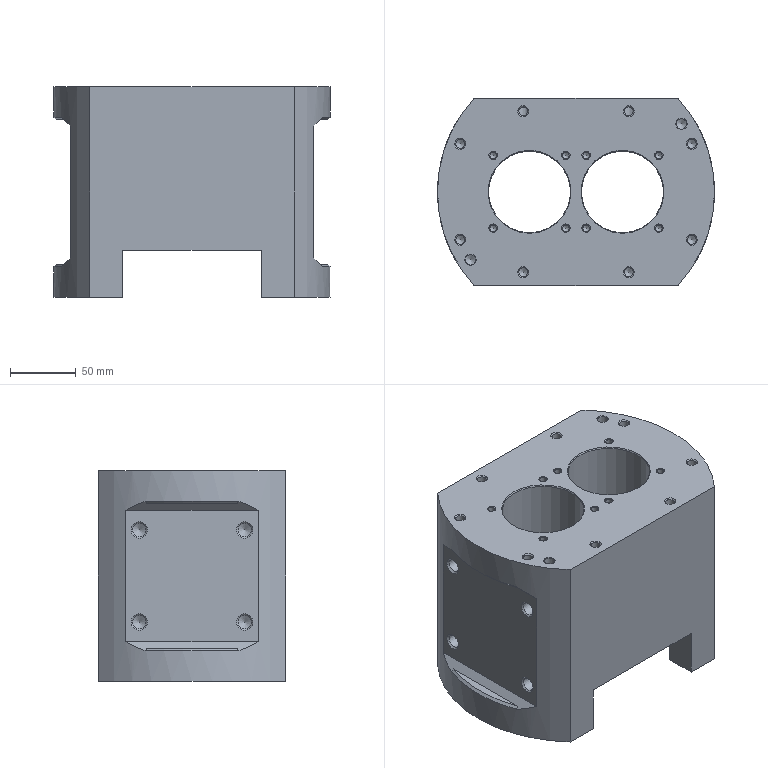NC program | NX | posted with a generic post | part box 210 x 142 x 160 mm
Lines 1 to 469 of 4730:
N10 G17 G21 G94 G90
(FLOOR_WALL_COPY_1_COPY_COPY , TOOL : D50)
N12 T02 M6
N14 G54
N16 G17 G0 G90 X25.097 Y36.47 B0. C0. S1200 M3
N18 G43 Z30. H2
N20 Z2.658
N22 G94 G1 Z-0.342 F1000.
N24 Y33.47
N26 Y-33.47 F2000.
N28 X-0.001
N30 Y33.47
N32 X-25.1
N34 Y-33.47
N36 Y-36.47
N38 Z2.658
N40 G0 Z30.
N42 X25.097 Y39.966
N44 Z2.316
N46 G1 Z-0.684 F1000.
N48 Y36.966
N50 Y-36.966 F2000.
N52 X-0.001
N54 Y36.966
N56 X-25.1
N58 Y-36.966
N60 Y-39.966
N62 Z2.316
N64 G0 Z30.
N66 X25.097 Y42.642
N68 Z1.974
N70 G1 Z-1.026 F1000.
N72 Y39.642
N74 Y-39.642 F2000.
N76 X-0.001
N78 Y39.642
N80 X-25.1
N82 Y-39.642
N84 Y-42.642
N86 Z1.974
N88 G0 Z30.
N90 X25.097 Y44.893
N92 Z1.632
N94 G1 Z-1.368 F1000.
N96 Y41.893
N98 Y-41.893 F2000.
N100 X-0.001
N102 Y41.893
N104 X-25.1
N106 Y-41.893
N108 Y-44.893
N110 Z1.632
N112 G0 Z30.
N114 X25.097 Y46.871
N116 Z1.29
N118 G1 Z-1.71 F1000.
N120 Y43.871
N122 Y-43.871 F2000.
N124 X-0.001
N126 Y43.871
N128 X-25.1
N130 Y-43.871
N132 Y-46.871
N134 Z1.29
N136 G0 Z30.
N138 X25.097 Y48.655
N140 Z0.948
N142 G1 Z-2.052 F1000.
N144 Y45.655
N146 Y-45.655 F2000.
N148 X-0.001
N150 Y45.655
N152 X-25.1
N154 Y-45.655
N156 Y-48.655
N158 Z0.948
N160 G0 Z30.
N162 X25.097 Y50.291
N164 Z0.607
N166 G1 Z-2.393 F1000.
N168 Y47.291
N170 Y-47.291 F2000.
N172 X-0.001
N174 Y47.291
N176 X-25.1
N178 Y-47.291
N180 Y-50.291
N182 Z0.607
N184 G0 Z30.
N186 X25.097 Y51.811
N188 Z0.265
N190 G1 Z-2.735 F1000.
N192 Y48.811
N194 Y-48.811 F2000.
N196 X-0.001
N198 Y48.811
N200 X-25.1
N202 Y-48.811
N204 Y-51.811
N206 Z0.265
N208 G0 Z30.
N210 X25.097 Y53.234
N212 Z-0.077
N214 G1 Z-3.077 F1000.
N216 Y50.234
N218 Y-50.234 F2000.
N220 X-0.001
N222 Y50.234
N224 X-25.1
N226 Y-50.234
N228 Y-53.234
N230 Z-0.077
N232 G0 Z30.
N234 X25.097 Y54.577
N236 Z-0.419
N238 G1 Z-3.419 F1000.
N240 Y51.577
N242 Y-51.577 F2000.
N244 X-0.001
N246 Y51.577
N248 X-25.1
N250 Y-51.577
N252 Y-54.577
N254 Z-0.419
N256 G0 Z30.
N258 X25.097 Y55.851
N260 Z-0.761
N262 G1 Z-3.761 F1000.
N264 Y52.851
N266 Y-52.851 F2000.
N268 X-0.001
N270 Y52.851
N272 X-25.1
N274 Y-52.851
N276 Y-55.851
N278 Z-0.761
N280 G0 Z30.
N282 X25.097 Y57.065
N284 Z-1.103
N286 G1 Z-4.103 F1000.
N288 Y54.065
N290 Y-54.065 F2000.
N292 X-0.001
N294 Y54.065
N296 X-25.1
N298 Y-54.065
N300 Y-57.065
N302 Z-1.103
N304 G0 Z30.
N306 X25.097 Y58.227
N308 Z-1.445
N310 G1 Z-4.445 F1000.
N312 Y55.227
N314 Y-55.227 F2000.
N316 X-0.001
N318 Y55.227
N320 X-25.1
N322 Y-55.227
N324 Y-58.227
N326 Z-1.445
N328 G0 Z30.
N330 X25.097 Y59.341
N332 Z-1.787
N334 G1 Z-4.787 F1000.
N336 Y56.341
N338 Y-56.341 F2000.
N340 X-0.001
N342 Y56.341
N344 X-25.1
N346 Y-56.341
N348 Y-59.341
N350 Z-1.787
N352 G0 Z30.
N354 X25.097 Y60.414
N356 Z-2.129
N358 G1 Z-5.129 F1000.
N360 Y57.414
N362 Y-57.414 F2000.
N364 X-0.001
N366 Y57.414
N368 X-25.1
N370 Y-57.414
N372 Y-60.414
N374 Z-2.129
N376 G0 Z30.
N378 X25.097 Y61.449
N380 Z-2.47
N382 G1 Z-5.47 F1000.
N384 Y58.449
N386 Y-58.449 F2000.
N388 X-0.001
N390 Y58.449
N392 X-25.1
N394 Y-58.449
N396 Y-61.449
N398 Z-2.47
N400 G0 Z30.
N402 X25.097 Y62.45
N404 Z-2.812
N406 G1 Z-5.812 F1000.
N408 Y59.45
N410 Y-59.45 F2000.
N412 X-0.001
N414 Y59.45
N416 X-25.1
N418 Y-59.45
N420 Y-62.45
N422 Z-2.812
N424 G0 Z30.
N426 X25.097 Y63.419
N428 Z-3.154
N430 G1 Z-6.154 F1000.
N432 Y60.419
N434 Y-60.419 F2000.
N436 X-0.001
N438 Y60.419
N440 X-25.1
N442 Y-60.419
N444 Y-63.419
N446 Z-3.154
N448 G0 Z30.
N450 X25.097 Y64.359
N452 Z-3.496
N454 G1 Z-6.496 F1000.
N456 Y61.359
N458 Y-61.359 F2000.
N460 X-0.001
N462 Y61.359
N464 X-25.1
N466 Y-61.359
N468 Y-64.359
N470 Z-3.496
N472 G0 Z30.
N474 X25.097 Y65.272
N476 Z-3.838
N478 G1 Z-6.838 F1000.
N480 Y62.272
N482 Y-62.272 F2000.
N484 X-0.001
N486 Y62.272
N488 X-25.1
N490 Y-62.272
N492 Y-65.272
N494 Z-3.838
N496 G0 Z30.
N498 X25.097 Y66.16
N500 Z-4.18
N502 G1 Z-7.18 F1000.
N504 Y63.16
N506 Y-63.16 F2000.
N508 X-0.001
N510 Y63.16
N512 X-25.1
N514 Y-63.16
N516 Y-66.16
N518 Z-4.18
N520 G0 Z30.
N522 X25.097 Y67.025
N524 Z-4.522
N526 G1 Z-7.522 F1000.
N528 Y64.025
N530 Y-64.025 F2000.
N532 X-0.001
N534 Y64.025
N536 X-25.1
N538 Y-64.025
N540 Y-67.025
N542 Z-4.522
N544 G0 Z30.
N546 X25.097 Y67.869
N548 Z-4.864
N550 G1 Z-7.864 F1000.
N552 Y64.869
N554 Y-64.869 F2000.
N556 X-0.001
N558 Y64.869
N560 X-25.1
N562 Y-64.869
N564 Y-67.869
N566 Z-4.864
N568 G0 Z30.
N570 X25.097 Y68.692
N572 Z-5.206
N574 G1 Z-8.206 F1000.
N576 Y65.692
N578 Y-65.692 F2000.
N580 X-0.001
N582 Y65.692
N584 X-25.1
N586 Y-65.692
N588 Y-68.692
N590 Z-5.206
N592 G0 Z30.
N594 X25.097 Y69.496
N596 Z-5.547
N598 G1 Z-8.547 F1000.
N600 Y66.496
N602 Y-66.496 F2000.
N604 X-0.001
N606 Y66.496
N608 X-25.1
N610 Y-66.496
N612 Y-69.496
N614 Z-5.547
N616 G0 Z30.
N618 X25.097 Y70.282
N620 Z-5.889
N622 G1 Z-8.889 F1000.
N624 Y67.282
N626 Y-67.282 F2000.
N628 X-0.001
N630 Y67.282
N632 X-25.1
N634 Y-67.282
N636 Y-70.282
N638 Z-5.889
N640 G0 Z30.
N642 X25.097 Y71.05
N644 Z-6.231
N646 G1 Z-9.231 F1000.
N648 Y68.05
N650 Y-68.05 F2000.
N652 X-0.001
N654 Y68.05
N656 X-25.1
N658 Y-68.05
N660 Y-71.05
N662 Z-6.231
N664 G0 Z30.
N666 X25.097 Y71.803
N668 Z-6.573
N670 G1 Z-9.573 F1000.
N672 Y68.803
N674 Y-68.803 F2000.
N676 X-0.001
N678 Y68.803
N680 X-25.1
N682 Y-68.803
N684 Y-71.803
N686 Z-6.573
N688 G0 Z30.
N690 X25.097 Y72.54
N692 Z-6.915
N694 G1 Z-9.915 F1000.
N696 Y69.54
N698 Y-69.54 F2000.
N700 X-0.001
N702 Y69.54
N704 X-25.1
N706 Y-69.54
N708 Y-72.54
N710 Z-6.915
N712 G0 Z30.
N714 X25.097 Y73.263
N716 Z-7.257
N718 G1 Z-10.257 F1000.
N720 Y70.263
N722 Y-70.263 F2000.
N724 X-0.001
N726 Y70.263
N728 X-25.1
N730 Y-70.263
N732 Y-73.263
N734 Z-7.257
N736 G0 Z30.
N738 X25.097 Y73.972
N740 Z-7.599
N742 G1 Z-10.599 F1000.
N744 Y70.972
N746 Y-70.972 F2000.
N748 X-0.001
N750 Y70.972
N752 X-25.1
N754 Y-70.972
N756 Y-73.972
N758 Z-7.599
N760 G0 Z30.
N762 X25.097 Y74.667
N764 Z-7.941
N766 G1 Z-10.941 F1000.
N768 Y71.667
N770 Y-71.667 F2000.
N772 X-0.001
N774 Y71.667
N776 X-25.1
N778 Y-71.667
N780 Y-74.667
N782 Z-7.941
N784 G0 Z30.
N786 X25.097 Y75.35
N788 Z-8.282
N790 G1 Z-11.282 F1000.
N792 Y72.35
N794 Y-72.35 F2000.
N796 X-0.001
N798 Y72.35
N800 X-25.1
N802 Y-72.35
N804 Y-75.35
N806 Z-8.282
N808 G0 Z30.
N810 X25.097 Y76.021
N812 Z-8.624
N814 G1 Z-11.624 F1000.
N816 Y73.021
N818 Y-73.021 F2000.
N820 X-0.001
N822 Y73.021
N824 X-25.1
N826 Y-73.021
N828 Y-76.021
N830 Z-8.624
N832 G0 Z30.
N834 X25.097 Y76.68
N836 Z-8.966
N838 G1 Z-11.966 F1000.
N840 Y73.68
N842 Y-73.68 F2000.
N844 X-0.001
N846 Y73.68
N848 X-25.1
N850 Y-73.68
N852 Y-76.68
N854 Z-8.966
N856 G0 Z30.
N858 X25.097 Y77.328
N860 Z-9.308
N862 G1 Z-12.308 F1000.
N864 Y74.328
N866 Y-74.328 F2000.
N868 X-0.001
N870 Y74.328
N872 X-25.1
N874 Y-74.328
N876 Y-77.328
N878 Z-9.308
N880 G0 Z30.
N882 X25.097 Y77.965
N884 Z-9.65
N886 G1 Z-12.65 F1000.
N888 Y74.965
N890 Y-74.965 F2000.
N892 X-0.001
N894 Y74.965
N896 X-25.1
N898 Y-74.965
N900 Y-77.965
N902 Z-9.65
N904 G0 Z30.
(FLOOR_WALL_COPY_COPY_COPY_COPY , TOOL : D50)
N906 X24.997 Y78.149 S2500
N908 Z-9.75
N910 G1 Z-12.75 F1000.
N912 Y75.149
N914 Y-75.149
N916 X-0.001
N918 Y75.149
N920 X-25.
N922 Y-75.149
N924 Y-78.149
N926 Z-9.75
N928 G0 Z30.
N930 M5